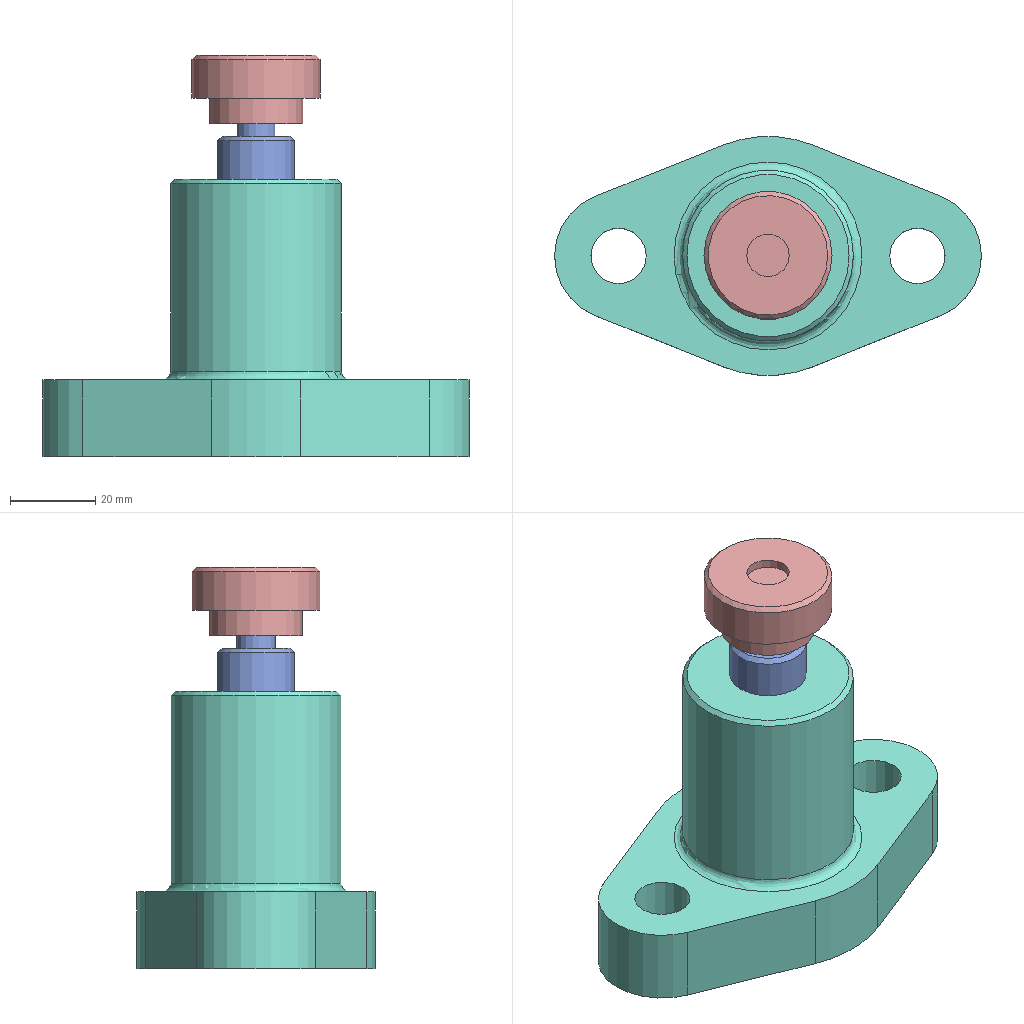Assembly | NX | 5 different items | 5 placed | box 100 x 56 x 94 mm
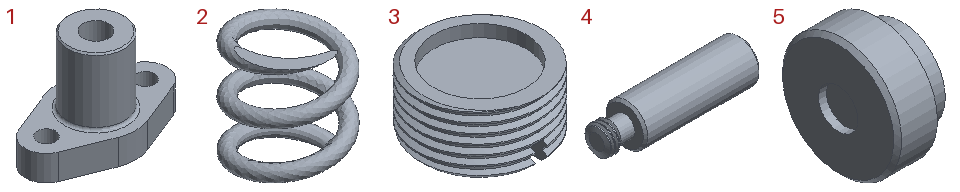Parts list (item | quantity | size | volume | features):
1 | x1 | 100 x 56 x 65 mm | 108287 mm3 | features EXTRUDE 4, DATUM_CSYS 2, BLEND 1, CHAMFER 1, HOLE PACKAGE 1, SIMPLE HOLE 1, SKETCH 1, SYMBOLIC_THREAD 1
2 | x1 | 13.997 x 13.994 x 17 mm | 306.817 mm3 | features DATUM_CSYS 2, SKETCH 2, DATUM_ON_PATH 1, EXTRUDE 1, HELIX 1, SKIN 1
3 | x1 | 20 x 20 x 10 mm | 2405 mm3 | features DATUM_CSYS 3, EXTRUDE 3, SKETCH 2, CHAMFER 1, THREADS 1
4 | x1 | 62 x 18 x 18 mm | 13574 mm3 | features DATUM_CSYS 2, CHAMFER 1, SKETCH 1, SWP104 1, THREADS 1
5 | x1 | 16 x 30 x 30 mm | 7540 mm3 | features DATUM_CSYS 2, CHAMFER 1, SKETCH 1, SWP104 1, THREADS 1
Mates (type | each side: item.copy, entity, surface, feature):
Fix | 1.1 component
Touch | 3.1 face cone Chamfer(4) | 1.1 face cylinder M20 x 1.5 Threaded Hole(5)
Parallel | 3.1 face plane Extrude(2) | 1.1 face plane Extrude(2)
Parallel | 3.1 face plane Extrude(7) | assembly plane
Touch | 3.1 face plane Extrude(2) | 1.1 face plane Extrude(2)
Touch | 2.1 face plane Extrude(5) | 3.1 face plane Extrude(3)
Fix | 2.1 component
Touch | 4.1 face cylinder Revolve(2) | 1.1 face cylinder Extrude(6)
Touch | 4.1 face plane Revolve(2) | 2.1 face plane Extrude(5)
Touch | 5.1 face cylinder Revolve(2) | 4.1 face cylinder Revolve(2)
Distance | 5.1 face plane Revolve(2) | 4.1 face plane Revolve(2)